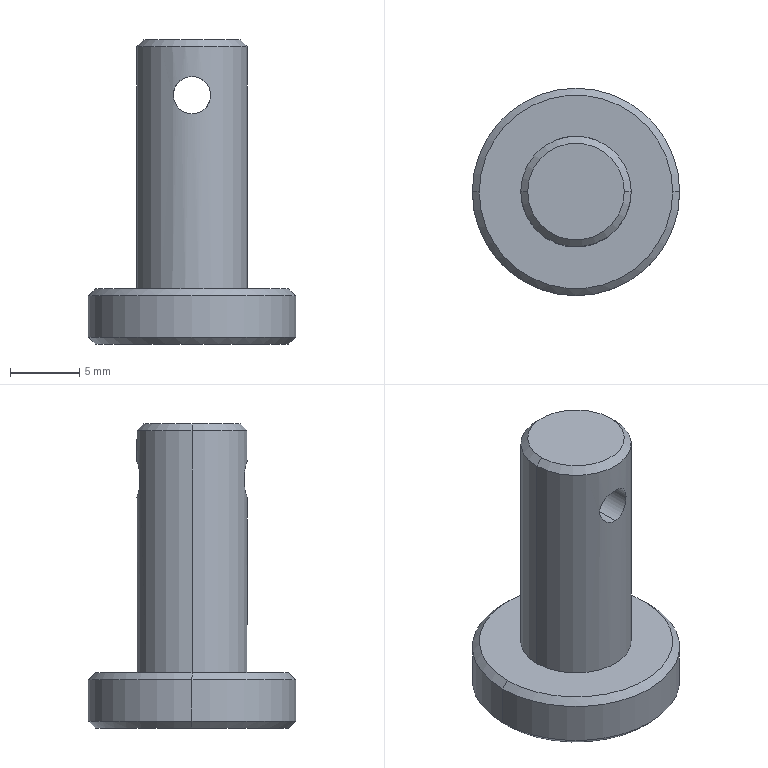Part | SolidWorks | features ICE 2, Chamfer 1, Extrusion 1 | 1 solid | 15 faces | box 15 x 15 x 22 mm | volume 1552 mm3 | cone 6 | cylinder 6 | plane 3 | commonest cylinder face diameters 2.7 x2 8 x2 15 x2
STEP:
#1=CARTESIAN_POINT('',(3.5,0.,18.));
#2=VERTEX_POINT('',#1);
#3=CARTESIAN_POINT('',(-3.5,0.,18.));
#4=VERTEX_POINT('',#3);
#5=CARTESIAN_POINT('',(0.,0.,18.));
#6=DIRECTION('',(0.,0.,1.));
#7=DIRECTION('',(1.,0.,0.));
#8=AXIS2_PLACEMENT_3D('',#5,#6,#7);
#9=CIRCLE('',#8,3.5);
#10=EDGE_CURVE('',#2,#4,#9,.T.);
#11=ORIENTED_EDGE('',*,*,#10,.F.);
#12=CARTESIAN_POINT('',(4.,0.,17.5));
#13=VERTEX_POINT('',#12);
#14=CARTESIAN_POINT('',(3.5,0.,18.));
#15=DIRECTION('',(0.7071,0.,-0.7071));
#16=VECTOR('',#15,1000.);
#17=LINE('',#14,#16);
#18=EDGE_CURVE('',#2,#13,#17,.T.);
#19=ORIENTED_EDGE('',*,*,#18,.T.);
#20=CARTESIAN_POINT('',(-4.,0.,17.5));
#21=VERTEX_POINT('',#20);
#22=CARTESIAN_POINT('',(0.,0.,17.5));
#23=DIRECTION('',(0.,0.,-1.));
#24=DIRECTION('',(1.,0.,0.));
#25=AXIS2_PLACEMENT_3D('',#22,#23,#24);
#26=CIRCLE('',#25,4.);
#27=EDGE_CURVE('',#21,#13,#26,.T.);
#28=ORIENTED_EDGE('',*,*,#27,.F.);
#29=CARTESIAN_POINT('',(-3.5,0.,18.));
#30=DIRECTION('',(-0.7071,0.,-0.7071));
#31=VECTOR('',#30,1000.);
#32=LINE('',#29,#31);
#33=EDGE_CURVE('',#4,#21,#32,.T.);
#34=ORIENTED_EDGE('',*,*,#33,.F.);
#35=EDGE_LOOP('',(#11,#19,#28,#34));
#36=FACE_OUTER_BOUND('',#35,.T.);
#37=CARTESIAN_POINT('',(0.,0.,18.));
#38=DIRECTION('',(0.,0.,-1.));
#39=DIRECTION('',(-1.,0.,0.));
#40=AXIS2_PLACEMENT_3D('',#37,#38,#39);
#41=CONICAL_SURFACE('',#40,3.5,0.7854);
#42=ADVANCED_FACE('',(#36),#41,.T.);
#43=CARTESIAN_POINT('',(7.,0.,0.));
#44=VERTEX_POINT('',#43);
#45=CARTESIAN_POINT('',(-7.,0.,0.));
#46=VERTEX_POINT('',#45);
#47=CARTESIAN_POINT('',(0.,0.,0.));
#48=DIRECTION('',(0.,0.,1.));
#49=DIRECTION('',(-1.,0.,0.));
#50=AXIS2_PLACEMENT_3D('',#47,#48,#49);
#51=CIRCLE('',#50,7.);
#52=EDGE_CURVE('',#44,#46,#51,.T.);
#53=ORIENTED_EDGE('',*,*,#52,.F.);
#54=CARTESIAN_POINT('',(7.5,0.,-0.5));
#55=VERTEX_POINT('',#54);
#56=CARTESIAN_POINT('',(7.5,0.,-0.5));
#57=DIRECTION('',(0.7071,0.,-0.7071));
#58=VECTOR('',#57,1000.);
#59=LINE('',#56,#58);
#60=EDGE_CURVE('',#44,#55,#59,.T.);
#61=ORIENTED_EDGE('',*,*,#60,.T.);
#62=CARTESIAN_POINT('',(-7.5,0.,-0.5));
#63=VERTEX_POINT('',#62);
#64=CARTESIAN_POINT('',(0.,0.,-0.5));
#65=DIRECTION('',(0.,0.,-1.));
#66=DIRECTION('',(-1.,0.,0.));
#67=AXIS2_PLACEMENT_3D('',#64,#65,#66);
#68=CIRCLE('',#67,7.5);
#69=EDGE_CURVE('',#63,#55,#68,.T.);
#70=ORIENTED_EDGE('',*,*,#69,.F.);
#71=CARTESIAN_POINT('',(-7.5,0.,-0.5));
#72=DIRECTION('',(-0.7071,0.,-0.7071));
#73=VECTOR('',#72,1000.);
#74=LINE('',#71,#73);
#75=EDGE_CURVE('',#46,#63,#74,.T.);
#76=ORIENTED_EDGE('',*,*,#75,.F.);
#77=EDGE_LOOP('',(#53,#61,#70,#76));
#78=FACE_OUTER_BOUND('',#77,.T.);
#79=CARTESIAN_POINT('',(0.,0.,-0.5));
#80=DIRECTION('',(0.,0.,-1.));
#81=DIRECTION('',(-1.,0.,0.));
#82=AXIS2_PLACEMENT_3D('',#79,#80,#81);
#83=CONICAL_SURFACE('',#82,7.5,0.7854);
#84=ADVANCED_FACE('',(#78),#83,.T.);
#85=CARTESIAN_POINT('',(-7.,0.,-4.));
#86=VERTEX_POINT('',#85);
#87=CARTESIAN_POINT('',(7.,0.,-4.));
#88=VERTEX_POINT('',#87);
#89=CARTESIAN_POINT('',(0.,0.,-4.));
#90=DIRECTION('',(0.,0.,-1.));
#91=DIRECTION('',(-1.,0.,0.));
#92=AXIS2_PLACEMENT_3D('',#89,#90,#91);
#93=CIRCLE('',#92,7.);
#94=EDGE_CURVE('',#86,#88,#93,.T.);
#95=ORIENTED_EDGE('',*,*,#94,.F.);
#96=CARTESIAN_POINT('',(-7.5,0.,-3.5));
#97=VERTEX_POINT('',#96);
#98=CARTESIAN_POINT('',(-7.,0.,-4.));
#99=DIRECTION('',(-0.7071,0.,0.7071));
#100=VECTOR('',#99,1000.);
#101=LINE('',#98,#100);
#102=EDGE_CURVE('',#86,#97,#101,.T.);
#103=ORIENTED_EDGE('',*,*,#102,.T.);
#104=CARTESIAN_POINT('',(7.5,0.,-3.5));
#105=VERTEX_POINT('',#104);
#106=CARTESIAN_POINT('',(0.,0.,-3.5));
#107=DIRECTION('',(0.,0.,1.));
#108=DIRECTION('',(-1.,0.,0.));
#109=AXIS2_PLACEMENT_3D('',#106,#107,#108);
#110=CIRCLE('',#109,7.5);
#111=EDGE_CURVE('',#105,#97,#110,.T.);
#112=ORIENTED_EDGE('',*,*,#111,.F.);
#113=CARTESIAN_POINT('',(7.,0.,-4.));
#114=DIRECTION('',(0.7071,0.,0.7071));
#115=VECTOR('',#114,1000.);
#116=LINE('',#113,#115);
#117=EDGE_CURVE('',#88,#105,#116,.T.);
#118=ORIENTED_EDGE('',*,*,#117,.F.);
#119=EDGE_LOOP('',(#95,#103,#112,#118));
#120=FACE_OUTER_BOUND('',#119,.T.);
#121=CARTESIAN_POINT('',(0.,0.,-4.));
#122=DIRECTION('',(0.,0.,1.));
#123=DIRECTION('',(1.,0.,0.));
#124=AXIS2_PLACEMENT_3D('',#121,#122,#123);
#125=CONICAL_SURFACE('',#124,7.,0.7854);
#126=ADVANCED_FACE('',(#120),#125,.T.);
#127=CARTESIAN_POINT('',(0.,-4.,12.65));
#128=VERTEX_POINT('',#127);
#129=CARTESIAN_POINT('',(0.,-4.,15.35));
#130=VERTEX_POINT('',#129);
#131=CARTESIAN_POINT('',(0.,-4.,12.65));
#132=CARTESIAN_POINT('',(-0.1771,-4.,12.65));
#133=CARTESIAN_POINT('',(-0.3558,-3.988,12.686));
#134=CARTESIAN_POINT('',(-0.6002,-3.956,12.788));
#135=CARTESIAN_POINT('',(-0.6792,-3.943,12.83));
#136=CARTESIAN_POINT('',(-0.8249,-3.915,12.928));
#137=CARTESIAN_POINT('',(-0.8925,-3.9,12.983));
#138=CARTESIAN_POINT('',(-1.079,-3.854,13.17));
#139=CARTESIAN_POINT('',(-1.178,-3.823,13.318));
#140=CARTESIAN_POINT('',(-1.281,-3.79,13.564));
#141=CARTESIAN_POINT('',(-1.306,-3.781,13.648));
#142=CARTESIAN_POINT('',(-1.341,-3.769,13.821));
#143=CARTESIAN_POINT('',(-1.35,-3.765,13.911));
#144=CARTESIAN_POINT('',(-1.35,-3.765,14.178));
#145=CARTESIAN_POINT('',(-1.314,-3.779,14.356));
#146=CARTESIAN_POINT('',(-1.179,-3.823,14.681));
#147=CARTESIAN_POINT('',(-1.078,-3.854,14.831));
#148=CARTESIAN_POINT('',(-0.8929,-3.9,15.016));
#149=CARTESIAN_POINT('',(-0.8239,-3.915,15.073));
#150=CARTESIAN_POINT('',(-0.6781,-3.943,15.171));
#151=CARTESIAN_POINT('',(-0.6009,-3.955,15.212));
#152=CARTESIAN_POINT('',(-0.4376,-3.977,15.28));
#153=CARTESIAN_POINT('',(-0.3516,-3.985,15.306));
#154=CARTESIAN_POINT('',(-0.1782,-3.997,15.341));
#155=CARTESIAN_POINT('',(-0.08989,-4.,15.35));
#156=CARTESIAN_POINT('',(0.,-4.,15.35));
#157=B_SPLINE_CURVE_WITH_KNOTS('',3,(#131,#132,#133,#134,#135,#136,#137,#138,#139,#140,#141,#142,#143,#144,#145,#146,#147,#148,#149,#150,#151,#152,#153,#154,#155,#156),.UNSPECIFIED.,.F.,.F.,(4,2,2,2,2,2,2,2,2,2,2,2,4),(0.004252,0.004784,0.005049,0.005315,0.005846,0.006112,0.006378,0.006909,0.007441,0.007706,0.007972,0.008238,0.008503),.UNSPECIFIED.);
#158=EDGE_CURVE('',#128,#130,#157,.T.);
#159=ORIENTED_EDGE('',*,*,#158,.F.);
#160=CARTESIAN_POINT('',(0.,4.,12.65));
#161=VERTEX_POINT('',#160);
#162=CARTESIAN_POINT('',(0.,-7.5,12.65));
#163=DIRECTION('',(0.,1.,0.));
#164=VECTOR('',#163,1000.);
#165=LINE('',#162,#164);
#166=EDGE_CURVE('',#128,#161,#165,.T.);
#167=ORIENTED_EDGE('',*,*,#166,.T.);
#168=CARTESIAN_POINT('',(0.,4.,15.35));
#169=VERTEX_POINT('',#168);
#170=CARTESIAN_POINT('',(0.,4.,15.35));
#171=CARTESIAN_POINT('',(-0.08991,4.,15.35));
#172=CARTESIAN_POINT('',(-0.1782,3.997,15.341));
#173=CARTESIAN_POINT('',(-0.3517,3.985,15.306));
#174=CARTESIAN_POINT('',(-0.4378,3.977,15.28));
#175=CARTESIAN_POINT('',(-0.6826,3.945,15.178));
#176=CARTESIAN_POINT('',(-0.8315,3.915,15.078));
#177=CARTESIAN_POINT('',(-1.079,3.854,14.831));
#178=CARTESIAN_POINT('',(-1.179,3.823,14.681));
#179=CARTESIAN_POINT('',(-1.314,3.779,14.357));
#180=CARTESIAN_POINT('',(-1.35,3.765,14.178));
#181=CARTESIAN_POINT('',(-1.35,3.765,13.912));
#182=CARTESIAN_POINT('',(-1.341,3.769,13.822));
#183=CARTESIAN_POINT('',(-1.306,3.781,13.648));
#184=CARTESIAN_POINT('',(-1.281,3.79,13.563));
#185=CARTESIAN_POINT('',(-1.178,3.823,13.317));
#186=CARTESIAN_POINT('',(-1.078,3.854,13.169));
#187=CARTESIAN_POINT('',(-0.8921,3.9,12.983));
#188=CARTESIAN_POINT('',(-0.8246,3.915,12.928));
#189=CARTESIAN_POINT('',(-0.6788,3.943,12.83));
#190=CARTESIAN_POINT('',(-0.5998,3.956,12.787));
#191=CARTESIAN_POINT('',(-0.3559,3.988,12.686));
#192=CARTESIAN_POINT('',(-0.1771,4.,12.65));
#193=CARTESIAN_POINT('',(0.,4.,12.65));
#194=B_SPLINE_CURVE_WITH_KNOTS('',3,(#170,#171,#172,#173,#174,#175,#176,#177,#178,#179,#180,#181,#182,#183,#184,#185,#186,#187,#188,#189,#190,#191,#192,#193),.UNSPECIFIED.,.F.,.F.,(4,2,2,2,2,2,2,2,2,2,2,4),(0.,0.0002658,0.0005315,0.001063,0.001595,0.002126,0.002392,0.002658,0.003189,0.003455,0.003721,0.004252),.UNSPECIFIED.);
#195=EDGE_CURVE('',#169,#161,#194,.T.);
#196=ORIENTED_EDGE('',*,*,#195,.F.);
#197=CARTESIAN_POINT('',(0.,-7.5,15.35));
#198=DIRECTION('',(0.,1.,0.));
#199=VECTOR('',#198,1000.);
#200=LINE('',#197,#199);
#201=EDGE_CURVE('',#130,#169,#200,.T.);
#202=ORIENTED_EDGE('',*,*,#201,.F.);
#203=EDGE_LOOP('',(#159,#167,#196,#202));
#204=FACE_OUTER_BOUND('',#203,.T.);
#205=CARTESIAN_POINT('',(0.,-7.5,14.));
#206=DIRECTION('',(0.,1.,0.));
#207=DIRECTION('',(0.,0.,1.));
#208=AXIS2_PLACEMENT_3D('',#205,#206,#207);
#209=CYLINDRICAL_SURFACE('',#208,1.35);
#210=ADVANCED_FACE('',(#204),#209,.F.);
#211=ORIENTED_EDGE('',*,*,#111,.T.);
#212=CARTESIAN_POINT('',(-7.5,0.,-4.));
#213=DIRECTION('',(0.,0.,1.));
#214=VECTOR('',#213,1000.);
#215=LINE('',#212,#214);
#216=EDGE_CURVE('',#97,#63,#215,.T.);
#217=ORIENTED_EDGE('',*,*,#216,.T.);
#218=ORIENTED_EDGE('',*,*,#69,.T.);
#219=CARTESIAN_POINT('',(7.5,0.,-4.));
#220=DIRECTION('',(0.,0.,1.));
#221=VECTOR('',#220,1000.);
#222=LINE('',#219,#221);
#223=EDGE_CURVE('',#105,#55,#222,.T.);
#224=ORIENTED_EDGE('',*,*,#223,.F.);
#225=EDGE_LOOP('',(#211,#217,#218,#224));
#226=FACE_OUTER_BOUND('',#225,.T.);
#227=CARTESIAN_POINT('',(0.,0.,-4.));
#228=DIRECTION('',(0.,0.,1.));
#229=DIRECTION('',(1.,0.,0.));
#230=AXIS2_PLACEMENT_3D('',#227,#228,#229);
#231=CYLINDRICAL_SURFACE('',#230,7.5);
#232=ADVANCED_FACE('',(#226),#231,.T.);
#233=ORIENTED_EDGE('',*,*,#195,.T.);
#234=CARTESIAN_POINT('',(0.,4.,12.65));
#235=CARTESIAN_POINT('',(0.1771,4.,12.65));
#236=CARTESIAN_POINT('',(0.3558,3.988,12.686));
#237=CARTESIAN_POINT('',(0.6002,3.956,12.788));
#238=CARTESIAN_POINT('',(0.6792,3.943,12.83));
#239=CARTESIAN_POINT('',(0.8249,3.915,12.928));
#240=CARTESIAN_POINT('',(0.8925,3.9,12.983));
#241=CARTESIAN_POINT('',(1.079,3.854,13.17));
#242=CARTESIAN_POINT('',(1.178,3.823,13.318));
#243=CARTESIAN_POINT('',(1.281,3.79,13.564));
#244=CARTESIAN_POINT('',(1.306,3.781,13.648));
#245=CARTESIAN_POINT('',(1.341,3.769,13.821));
#246=CARTESIAN_POINT('',(1.35,3.765,13.911));
#247=CARTESIAN_POINT('',(1.35,3.765,14.178));
#248=CARTESIAN_POINT('',(1.314,3.779,14.356));
#249=CARTESIAN_POINT('',(1.179,3.823,14.681));
#250=CARTESIAN_POINT('',(1.078,3.854,14.831));
#251=CARTESIAN_POINT('',(0.8929,3.9,15.016));
#252=CARTESIAN_POINT('',(0.8239,3.915,15.073));
#253=CARTESIAN_POINT('',(0.6781,3.943,15.171));
#254=CARTESIAN_POINT('',(0.6009,3.955,15.212));
#255=CARTESIAN_POINT('',(0.4376,3.977,15.28));
#256=CARTESIAN_POINT('',(0.3516,3.985,15.306));
#257=CARTESIAN_POINT('',(0.1782,3.997,15.341));
#258=CARTESIAN_POINT('',(0.08989,4.,15.35));
#259=CARTESIAN_POINT('',(0.,4.,15.35));
#260=B_SPLINE_CURVE_WITH_KNOTS('',3,(#234,#235,#236,#237,#238,#239,#240,#241,#242,#243,#244,#245,#246,#247,#248,#249,#250,#251,#252,#253,#254,#255,#256,#257,#258,#259),.UNSPECIFIED.,.F.,.F.,(4,2,2,2,2,2,2,2,2,2,2,2,4),(0.004252,0.004784,0.005049,0.005315,0.005846,0.006112,0.006378,0.006909,0.007441,0.007706,0.007972,0.008238,0.008503),.UNSPECIFIED.);
#261=EDGE_CURVE('',#161,#169,#260,.T.);
#262=ORIENTED_EDGE('',*,*,#261,.T.);
#263=EDGE_LOOP('',(#233,#262));
#264=FACE_BOUND('',#263,.T.);
#265=ORIENTED_EDGE('',*,*,#27,.T.);
#266=CARTESIAN_POINT('',(4.,0.,0.));
#267=VERTEX_POINT('',#266);
#268=CARTESIAN_POINT('',(4.,0.,18.));
#269=DIRECTION('',(0.,0.,-1.));
#270=VECTOR('',#269,1000.);
#271=LINE('',#268,#270);
#272=EDGE_CURVE('',#13,#267,#271,.T.);
#273=ORIENTED_EDGE('',*,*,#272,.T.);
#274=CARTESIAN_POINT('',(-4.,0.,0.));
#275=VERTEX_POINT('',#274);
#276=CARTESIAN_POINT('',(0.,0.,0.));
#277=DIRECTION('',(0.,0.,1.));
#278=DIRECTION('',(1.,0.,0.));
#279=AXIS2_PLACEMENT_3D('',#276,#277,#278);
#280=CIRCLE('',#279,4.);
#281=EDGE_CURVE('',#267,#275,#280,.T.);
#282=ORIENTED_EDGE('',*,*,#281,.T.);
#283=CARTESIAN_POINT('',(-4.,0.,18.));
#284=DIRECTION('',(0.,0.,-1.));
#285=VECTOR('',#284,1000.);
#286=LINE('',#283,#285);
#287=EDGE_CURVE('',#21,#275,#286,.T.);
#288=ORIENTED_EDGE('',*,*,#287,.F.);
#289=EDGE_LOOP('',(#265,#273,#282,#288));
#290=FACE_OUTER_BOUND('',#289,.T.);
#291=CARTESIAN_POINT('',(0.,0.,18.));
#292=DIRECTION('',(0.,0.,-1.));
#293=DIRECTION('',(-1.,0.,0.));
#294=AXIS2_PLACEMENT_3D('',#291,#292,#293);
#295=CYLINDRICAL_SURFACE('',#294,4.);
#296=ADVANCED_FACE('',(#264,#290),#295,.T.);
#297=ORIENTED_EDGE('',*,*,#272,.F.);
#298=CARTESIAN_POINT('',(0.,0.,17.5));
#299=DIRECTION('',(0.,0.,-1.));
#300=DIRECTION('',(1.,0.,0.));
#301=AXIS2_PLACEMENT_3D('',#298,#299,#300);
#302=CIRCLE('',#301,4.);
#303=EDGE_CURVE('',#13,#21,#302,.T.);
#304=ORIENTED_EDGE('',*,*,#303,.T.);
#305=ORIENTED_EDGE('',*,*,#287,.T.);
#306=CARTESIAN_POINT('',(0.,0.,0.));
#307=DIRECTION('',(0.,0.,1.));
#308=DIRECTION('',(1.,0.,0.));
#309=AXIS2_PLACEMENT_3D('',#306,#307,#308);
#310=CIRCLE('',#309,4.);
#311=EDGE_CURVE('',#275,#267,#310,.T.);
#312=ORIENTED_EDGE('',*,*,#311,.T.);
#313=EDGE_LOOP('',(#297,#304,#305,#312));
#314=FACE_OUTER_BOUND('',#313,.T.);
#315=CARTESIAN_POINT('',(0.,-4.,15.35));
#316=CARTESIAN_POINT('',(0.08991,-4.,15.35));
#317=CARTESIAN_POINT('',(0.1782,-3.997,15.341));
#318=CARTESIAN_POINT('',(0.3517,-3.985,15.306));
#319=CARTESIAN_POINT('',(0.4378,-3.977,15.28));
#320=CARTESIAN_POINT('',(0.6826,-3.945,15.178));
#321=CARTESIAN_POINT('',(0.8315,-3.915,15.078));
#322=CARTESIAN_POINT('',(1.079,-3.854,14.831));
#323=CARTESIAN_POINT('',(1.179,-3.823,14.681));
#324=CARTESIAN_POINT('',(1.314,-3.779,14.357));
#325=CARTESIAN_POINT('',(1.35,-3.765,14.178));
#326=CARTESIAN_POINT('',(1.35,-3.765,13.912));
#327=CARTESIAN_POINT('',(1.341,-3.769,13.822));
#328=CARTESIAN_POINT('',(1.306,-3.781,13.648));
#329=CARTESIAN_POINT('',(1.281,-3.79,13.563));
#330=CARTESIAN_POINT('',(1.178,-3.823,13.317));
#331=CARTESIAN_POINT('',(1.078,-3.854,13.169));
#332=CARTESIAN_POINT('',(0.8921,-3.9,12.983));
#333=CARTESIAN_POINT('',(0.8246,-3.915,12.928));
#334=CARTESIAN_POINT('',(0.6788,-3.943,12.83));
#335=CARTESIAN_POINT('',(0.5998,-3.956,12.787));
#336=CARTESIAN_POINT('',(0.3559,-3.988,12.686));
#337=CARTESIAN_POINT('',(0.1771,-4.,12.65));
#338=CARTESIAN_POINT('',(0.,-4.,12.65));
#339=B_SPLINE_CURVE_WITH_KNOTS('',3,(#315,#316,#317,#318,#319,#320,#321,#322,#323,#324,#325,#326,#327,#328,#329,#330,#331,#332,#333,#334,#335,#336,#337,#338),.UNSPECIFIED.,.F.,.F.,(4,2,2,2,2,2,2,2,2,2,2,4),(0.,0.0002658,0.0005315,0.001063,0.001595,0.002126,0.002392,0.002658,0.003189,0.003455,0.003721,0.004252),.UNSPECIFIED.);
#340=EDGE_CURVE('',#130,#128,#339,.T.);
#341=ORIENTED_EDGE('',*,*,#340,.T.);
#342=ORIENTED_EDGE('',*,*,#158,.T.);
#343=EDGE_LOOP('',(#341,#342));
#344=FACE_BOUND('',#343,.T.);
#345=CARTESIAN_POINT('',(0.,0.,18.));
#346=DIRECTION('',(0.,0.,-1.));
#347=DIRECTION('',(-1.,0.,0.));
#348=AXIS2_PLACEMENT_3D('',#345,#346,#347);
#349=CYLINDRICAL_SURFACE('',#348,4.);
#350=ADVANCED_FACE('',(#314,#344),#349,.T.);
#351=CARTESIAN_POINT('',(0.,0.,18.));
#352=DIRECTION('',(0.,0.,1.));
#353=DIRECTION('',(1.,0.,0.));
#354=AXIS2_PLACEMENT_3D('',#351,#352,#353);
#355=CIRCLE('',#354,3.5);
#356=EDGE_CURVE('',#4,#2,#355,.T.);
#357=ORIENTED_EDGE('',*,*,#356,.T.);
#358=ORIENTED_EDGE('',*,*,#10,.T.);
#359=EDGE_LOOP('',(#357,#358));
#360=FACE_OUTER_BOUND('',#359,.T.);
#361=CARTESIAN_POINT('',(0.,0.,18.));
#362=DIRECTION('',(0.,0.,1.));
#363=DIRECTION('',(1.,0.,0.));
#364=AXIS2_PLACEMENT_3D('',#361,#362,#363);
#365=PLANE('',#364);
#366=ADVANCED_FACE('',(#360),#365,.T.);
#367=ORIENTED_EDGE('',*,*,#216,.F.);
#368=CARTESIAN_POINT('',(0.,0.,-3.5));
#369=DIRECTION('',(0.,0.,1.));
#370=DIRECTION('',(-1.,0.,0.));
#371=AXIS2_PLACEMENT_3D('',#368,#369,#370);
#372=CIRCLE('',#371,7.5);
#373=EDGE_CURVE('',#97,#105,#372,.T.);
#374=ORIENTED_EDGE('',*,*,#373,.T.);
#375=ORIENTED_EDGE('',*,*,#223,.T.);
#376=CARTESIAN_POINT('',(0.,0.,-0.5));
#377=DIRECTION('',(0.,0.,-1.));
#378=DIRECTION('',(-1.,0.,0.));
#379=AXIS2_PLACEMENT_3D('',#376,#377,#378);
#380=CIRCLE('',#379,7.5);
#381=EDGE_CURVE('',#55,#63,#380,.T.);
#382=ORIENTED_EDGE('',*,*,#381,.T.);
#383=EDGE_LOOP('',(#367,#374,#375,#382));
#384=FACE_OUTER_BOUND('',#383,.T.);
#385=CARTESIAN_POINT('',(0.,0.,-4.));
#386=DIRECTION('',(0.,0.,1.));
#387=DIRECTION('',(1.,0.,0.));
#388=AXIS2_PLACEMENT_3D('',#385,#386,#387);
#389=CYLINDRICAL_SURFACE('',#388,7.5);
#390=ADVANCED_FACE('',(#384),#389,.T.);
#391=CARTESIAN_POINT('',(0.,0.,-4.));
#392=DIRECTION('',(0.,0.,-1.));
#393=DIRECTION('',(-1.,0.,0.));
#394=AXIS2_PLACEMENT_3D('',#391,#392,#393);
#395=CIRCLE('',#394,7.);
#396=EDGE_CURVE('',#88,#86,#395,.T.);
#397=ORIENTED_EDGE('',*,*,#396,.T.);
#398=ORIENTED_EDGE('',*,*,#94,.T.);
#399=EDGE_LOOP('',(#397,#398));
#400=FACE_OUTER_BOUND('',#399,.T.);
#401=CARTESIAN_POINT('',(0.,0.,-4.));
#402=DIRECTION('',(0.,0.,-1.));
#403=DIRECTION('',(-1.,0.,0.));
#404=AXIS2_PLACEMENT_3D('',#401,#402,#403);
#405=PLANE('',#404);
#406=ADVANCED_FACE('',(#400),#405,.T.);
#407=CARTESIAN_POINT('',(0.,0.,0.));
#408=DIRECTION('',(0.,0.,1.));
#409=DIRECTION('',(-1.,0.,0.));
#410=AXIS2_PLACEMENT_3D('',#407,#408,#409);
#411=CIRCLE('',#410,7.);
#412=EDGE_CURVE('',#46,#44,#411,.T.);
#413=ORIENTED_EDGE('',*,*,#412,.T.);
#414=ORIENTED_EDGE('',*,*,#52,.T.);
#415=EDGE_LOOP('',(#413,#414));
#416=FACE_OUTER_BOUND('',#415,.T.);
#417=ORIENTED_EDGE('',*,*,#311,.F.);
#418=ORIENTED_EDGE('',*,*,#281,.F.);
#419=EDGE_LOOP('',(#417,#418));
#420=FACE_BOUND('',#419,.T.);
#421=CARTESIAN_POINT('',(0.,0.,0.));
#422=DIRECTION('',(0.,0.,-1.));
#423=DIRECTION('',(-1.,0.,0.));
#424=AXIS2_PLACEMENT_3D('',#421,#422,#423);
#425=PLANE('',#424);
#426=ADVANCED_FACE('',(#416,#420),#425,.F.);
#427=ORIENTED_EDGE('',*,*,#166,.F.);
#428=ORIENTED_EDGE('',*,*,#340,.F.);
#429=ORIENTED_EDGE('',*,*,#201,.T.);
#430=ORIENTED_EDGE('',*,*,#261,.F.);
#431=EDGE_LOOP('',(#427,#428,#429,#430));
#432=FACE_OUTER_BOUND('',#431,.T.);
#433=CARTESIAN_POINT('',(0.,-7.5,14.));
#434=DIRECTION('',(0.,1.,0.));
#435=DIRECTION('',(0.,0.,1.));
#436=AXIS2_PLACEMENT_3D('',#433,#434,#435);
#437=CYLINDRICAL_SURFACE('',#436,1.35);
#438=ADVANCED_FACE('',(#432),#437,.F.);
#439=ORIENTED_EDGE('',*,*,#102,.F.);
#440=ORIENTED_EDGE('',*,*,#396,.F.);
#441=ORIENTED_EDGE('',*,*,#117,.T.);
#442=ORIENTED_EDGE('',*,*,#373,.F.);
#443=EDGE_LOOP('',(#439,#440,#441,#442));
#444=FACE_OUTER_BOUND('',#443,.T.);
#445=CARTESIAN_POINT('',(0.,0.,-4.));
#446=DIRECTION('',(0.,0.,1.));
#447=DIRECTION('',(1.,0.,0.));
#448=AXIS2_PLACEMENT_3D('',#445,#446,#447);
#449=CONICAL_SURFACE('',#448,7.,0.7854);
#450=ADVANCED_FACE('',(#444),#449,.T.);
#451=ORIENTED_EDGE('',*,*,#60,.F.);
#452=ORIENTED_EDGE('',*,*,#412,.F.);
#453=ORIENTED_EDGE('',*,*,#75,.T.);
#454=ORIENTED_EDGE('',*,*,#381,.F.);
#455=EDGE_LOOP('',(#451,#452,#453,#454));
#456=FACE_OUTER_BOUND('',#455,.T.);
#457=CARTESIAN_POINT('',(0.,0.,-0.5));
#458=DIRECTION('',(0.,0.,-1.));
#459=DIRECTION('',(-1.,0.,0.));
#460=AXIS2_PLACEMENT_3D('',#457,#458,#459);
#461=CONICAL_SURFACE('',#460,7.5,0.7854);
#462=ADVANCED_FACE('',(#456),#461,.T.);
#463=ORIENTED_EDGE('',*,*,#18,.F.);
#464=ORIENTED_EDGE('',*,*,#356,.F.);
#465=ORIENTED_EDGE('',*,*,#33,.T.);
#466=ORIENTED_EDGE('',*,*,#303,.F.);
#467=EDGE_LOOP('',(#463,#464,#465,#466));
#468=FACE_OUTER_BOUND('',#467,.T.);
#469=CARTESIAN_POINT('',(0.,0.,18.));
#470=DIRECTION('',(0.,0.,-1.));
#471=DIRECTION('',(-1.,0.,0.));
#472=AXIS2_PLACEMENT_3D('',#469,#470,#471);
#473=CONICAL_SURFACE('',#472,3.5,0.7854);
#474=ADVANCED_FACE('',(#468),#473,.T.);
#475=CLOSED_SHELL('',(#42,#84,#126,#210,#232,#296,#350,#366,#390,#406,#426,#438,#450,#462,#474));
#476=MANIFOLD_SOLID_BREP('',#475);
#477=CARTESIAN_POINT('',(0.,0.,0.));
#478=DIRECTION('',(0.,0.,1.));
#479=DIRECTION('',(1.,0.,0.));
#480=AXIS2_PLACEMENT_3D('',#477,#478,#479);
#481=(LENGTH_UNIT()NAMED_UNIT(*)SI_UNIT(.MILLI.,.METRE.));
#482=UNCERTAINTY_MEASURE_WITH_UNIT(LENGTH_MEASURE(0.00001),#481,'','');
#483=(NAMED_UNIT(*)PLANE_ANGLE_UNIT()SI_UNIT($,.RADIAN.));
#484=(NAMED_UNIT(*)SI_UNIT($,.STERADIAN.)SOLID_ANGLE_UNIT());
#485=(GEOMETRIC_REPRESENTATION_CONTEXT(3)GLOBAL_UNCERTAINTY_ASSIGNED_CONTEXT((#482))GLOBAL_UNIT_ASSIGNED_CONTEXT((#481,#483,#484))REPRESENTATION_CONTEXT('',''));
#486=ADVANCED_BREP_SHAPE_REPRESENTATION('',(#476,#480),#485);